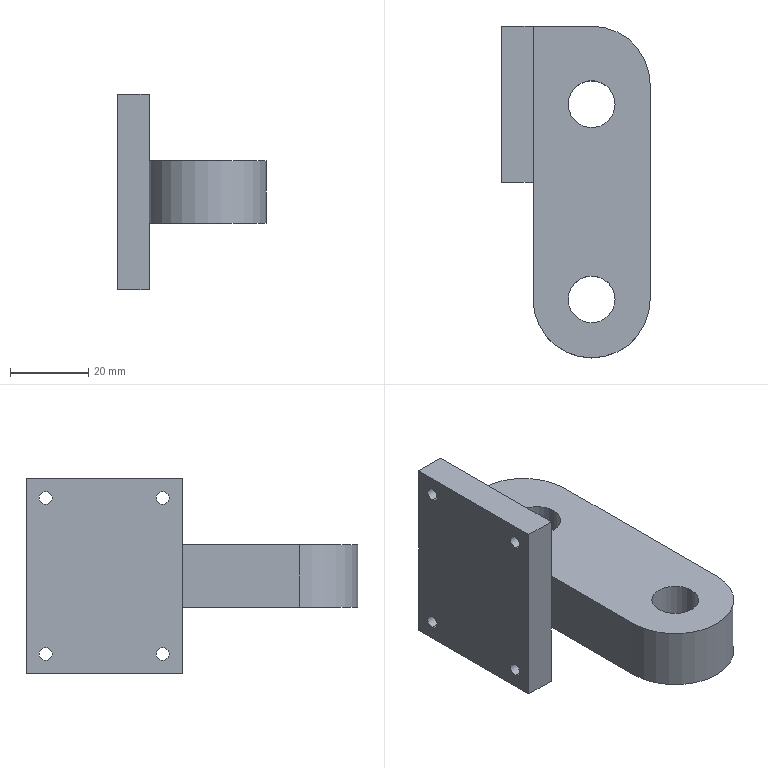Part | STEP file | X77-03303 | 1 solid | 25 faces | box 38 x 85 x 50 mm | volume 50589 mm3 | cylinder 14 | plane 11 | commonest cylinder face diameters 3.3 x8 12 x4 30 x2
STEP:
#1=CARTESIAN_POINT('',(98.602,105.281,26.35));
#2=VERTEX_POINT('',#1);
#3=CARTESIAN_POINT('',(98.602,105.281,29.65));
#4=VERTEX_POINT('',#3);
#5=CARTESIAN_POINT('',(98.602,105.281,28.));
#6=DIRECTION('',(-1.,0.,0.));
#7=DIRECTION('',(0.,0.,1.));
#8=AXIS2_PLACEMENT_3D('',#5,#6,#7);
#9=CIRCLE('',#8,1.65);
#10=EDGE_CURVE('',#2,#4,#9,.T.);
#11=ORIENTED_EDGE('',*,*,#10,.F.);
#12=CARTESIAN_POINT('',(90.602,105.281,26.35));
#13=VERTEX_POINT('',#12);
#14=CARTESIAN_POINT('',(90.602,105.281,26.35));
#15=DIRECTION('',(-1.,0.,0.));
#16=VECTOR('',#15,1000.);
#17=LINE('',#14,#16);
#18=EDGE_CURVE('',#2,#13,#17,.T.);
#19=ORIENTED_EDGE('',*,*,#18,.T.);
#20=CARTESIAN_POINT('',(90.602,105.281,29.65));
#21=VERTEX_POINT('',#20);
#22=CARTESIAN_POINT('',(90.602,105.281,28.));
#23=DIRECTION('',(-1.,0.,0.));
#24=DIRECTION('',(0.,0.,1.));
#25=AXIS2_PLACEMENT_3D('',#22,#23,#24);
#26=CIRCLE('',#25,1.65);
#27=EDGE_CURVE('',#13,#21,#26,.T.);
#28=ORIENTED_EDGE('',*,*,#27,.T.);
#29=CARTESIAN_POINT('',(90.602,105.281,29.65));
#30=DIRECTION('',(-1.,0.,0.));
#31=VECTOR('',#30,1000.);
#32=LINE('',#29,#31);
#33=EDGE_CURVE('',#4,#21,#32,.T.);
#34=ORIENTED_EDGE('',*,*,#33,.F.);
#35=EDGE_LOOP('',(#11,#19,#28,#34));
#36=FACE_OUTER_BOUND('',#35,.T.);
#37=CARTESIAN_POINT('',(90.602,105.281,28.));
#38=DIRECTION('',(-1.,0.,0.));
#39=DIRECTION('',(0.,0.,1.));
#40=AXIS2_PLACEMENT_3D('',#37,#38,#39);
#41=CYLINDRICAL_SURFACE('',#40,1.65);
#42=ADVANCED_FACE('',(#36),#41,.F.);
#43=CARTESIAN_POINT('',(98.602,105.281,-13.65));
#44=VERTEX_POINT('',#43);
#45=CARTESIAN_POINT('',(98.602,105.281,-10.35));
#46=VERTEX_POINT('',#45);
#47=CARTESIAN_POINT('',(98.602,105.281,-12.));
#48=DIRECTION('',(-1.,0.,0.));
#49=DIRECTION('',(0.,0.,1.));
#50=AXIS2_PLACEMENT_3D('',#47,#48,#49);
#51=CIRCLE('',#50,1.65);
#52=EDGE_CURVE('',#44,#46,#51,.T.);
#53=ORIENTED_EDGE('',*,*,#52,.F.);
#54=CARTESIAN_POINT('',(90.602,105.281,-13.65));
#55=VERTEX_POINT('',#54);
#56=CARTESIAN_POINT('',(90.602,105.281,-13.65));
#57=DIRECTION('',(-1.,0.,0.));
#58=VECTOR('',#57,1000.);
#59=LINE('',#56,#58);
#60=EDGE_CURVE('',#44,#55,#59,.T.);
#61=ORIENTED_EDGE('',*,*,#60,.T.);
#62=CARTESIAN_POINT('',(90.602,105.281,-10.35));
#63=VERTEX_POINT('',#62);
#64=CARTESIAN_POINT('',(90.602,105.281,-12.));
#65=DIRECTION('',(-1.,0.,0.));
#66=DIRECTION('',(0.,0.,1.));
#67=AXIS2_PLACEMENT_3D('',#64,#65,#66);
#68=CIRCLE('',#67,1.65);
#69=EDGE_CURVE('',#55,#63,#68,.T.);
#70=ORIENTED_EDGE('',*,*,#69,.T.);
#71=CARTESIAN_POINT('',(90.602,105.281,-10.35));
#72=DIRECTION('',(-1.,0.,0.));
#73=VECTOR('',#72,1000.);
#74=LINE('',#71,#73);
#75=EDGE_CURVE('',#46,#63,#74,.T.);
#76=ORIENTED_EDGE('',*,*,#75,.F.);
#77=EDGE_LOOP('',(#53,#61,#70,#76));
#78=FACE_OUTER_BOUND('',#77,.T.);
#79=CARTESIAN_POINT('',(90.602,105.281,-12.));
#80=DIRECTION('',(-1.,0.,0.));
#81=DIRECTION('',(0.,0.,1.));
#82=AXIS2_PLACEMENT_3D('',#79,#80,#81);
#83=CYLINDRICAL_SURFACE('',#82,1.65);
#84=ADVANCED_FACE('',(#78),#83,.F.);
#85=CARTESIAN_POINT('',(98.602,75.281,26.35));
#86=VERTEX_POINT('',#85);
#87=CARTESIAN_POINT('',(98.602,75.281,29.65));
#88=VERTEX_POINT('',#87);
#89=CARTESIAN_POINT('',(98.602,75.281,28.));
#90=DIRECTION('',(-1.,0.,0.));
#91=DIRECTION('',(0.,0.,1.));
#92=AXIS2_PLACEMENT_3D('',#89,#90,#91);
#93=CIRCLE('',#92,1.65);
#94=EDGE_CURVE('',#86,#88,#93,.T.);
#95=ORIENTED_EDGE('',*,*,#94,.F.);
#96=CARTESIAN_POINT('',(90.602,75.281,26.35));
#97=VERTEX_POINT('',#96);
#98=CARTESIAN_POINT('',(90.602,75.281,26.35));
#99=DIRECTION('',(-1.,0.,0.));
#100=VECTOR('',#99,1000.);
#101=LINE('',#98,#100);
#102=EDGE_CURVE('',#86,#97,#101,.T.);
#103=ORIENTED_EDGE('',*,*,#102,.T.);
#104=CARTESIAN_POINT('',(90.602,75.281,29.65));
#105=VERTEX_POINT('',#104);
#106=CARTESIAN_POINT('',(90.602,75.281,28.));
#107=DIRECTION('',(-1.,0.,0.));
#108=DIRECTION('',(0.,0.,1.));
#109=AXIS2_PLACEMENT_3D('',#106,#107,#108);
#110=CIRCLE('',#109,1.65);
#111=EDGE_CURVE('',#97,#105,#110,.T.);
#112=ORIENTED_EDGE('',*,*,#111,.T.);
#113=CARTESIAN_POINT('',(90.602,75.281,29.65));
#114=DIRECTION('',(-1.,0.,0.));
#115=VECTOR('',#114,1000.);
#116=LINE('',#113,#115);
#117=EDGE_CURVE('',#88,#105,#116,.T.);
#118=ORIENTED_EDGE('',*,*,#117,.F.);
#119=EDGE_LOOP('',(#95,#103,#112,#118));
#120=FACE_OUTER_BOUND('',#119,.T.);
#121=CARTESIAN_POINT('',(90.602,75.281,28.));
#122=DIRECTION('',(-1.,0.,0.));
#123=DIRECTION('',(0.,0.,1.));
#124=AXIS2_PLACEMENT_3D('',#121,#122,#123);
#125=CYLINDRICAL_SURFACE('',#124,1.65);
#126=ADVANCED_FACE('',(#120),#125,.F.);
#127=CARTESIAN_POINT('',(98.602,75.281,-13.65));
#128=VERTEX_POINT('',#127);
#129=CARTESIAN_POINT('',(98.602,75.281,-10.35));
#130=VERTEX_POINT('',#129);
#131=CARTESIAN_POINT('',(98.602,75.281,-12.));
#132=DIRECTION('',(-1.,0.,0.));
#133=DIRECTION('',(0.,0.,1.));
#134=AXIS2_PLACEMENT_3D('',#131,#132,#133);
#135=CIRCLE('',#134,1.65);
#136=EDGE_CURVE('',#128,#130,#135,.T.);
#137=ORIENTED_EDGE('',*,*,#136,.F.);
#138=CARTESIAN_POINT('',(90.602,75.281,-13.65));
#139=VERTEX_POINT('',#138);
#140=CARTESIAN_POINT('',(90.602,75.281,-13.65));
#141=DIRECTION('',(-1.,0.,0.));
#142=VECTOR('',#141,1000.);
#143=LINE('',#140,#142);
#144=EDGE_CURVE('',#128,#139,#143,.T.);
#145=ORIENTED_EDGE('',*,*,#144,.T.);
#146=CARTESIAN_POINT('',(90.602,75.281,-10.35));
#147=VERTEX_POINT('',#146);
#148=CARTESIAN_POINT('',(90.602,75.281,-12.));
#149=DIRECTION('',(-1.,0.,0.));
#150=DIRECTION('',(0.,0.,1.));
#151=AXIS2_PLACEMENT_3D('',#148,#149,#150);
#152=CIRCLE('',#151,1.65);
#153=EDGE_CURVE('',#139,#147,#152,.T.);
#154=ORIENTED_EDGE('',*,*,#153,.T.);
#155=CARTESIAN_POINT('',(90.602,75.281,-10.35));
#156=DIRECTION('',(-1.,0.,0.));
#157=VECTOR('',#156,1000.);
#158=LINE('',#155,#157);
#159=EDGE_CURVE('',#130,#147,#158,.T.);
#160=ORIENTED_EDGE('',*,*,#159,.F.);
#161=EDGE_LOOP('',(#137,#145,#154,#160));
#162=FACE_OUTER_BOUND('',#161,.T.);
#163=CARTESIAN_POINT('',(90.602,75.281,-12.));
#164=DIRECTION('',(-1.,0.,0.));
#165=DIRECTION('',(0.,0.,1.));
#166=AXIS2_PLACEMENT_3D('',#163,#164,#165);
#167=CYLINDRICAL_SURFACE('',#166,1.65);
#168=ADVANCED_FACE('',(#162),#167,.F.);
#169=CARTESIAN_POINT('',(107.602,90.281,16.));
#170=VERTEX_POINT('',#169);
#171=CARTESIAN_POINT('',(119.602,90.281,16.));
#172=VERTEX_POINT('',#171);
#173=CARTESIAN_POINT('',(113.602,90.281,16.));
#174=DIRECTION('',(0.,0.,1.));
#175=DIRECTION('',(1.,0.,0.));
#176=AXIS2_PLACEMENT_3D('',#173,#174,#175);
#177=CIRCLE('',#176,6.);
#178=EDGE_CURVE('',#170,#172,#177,.T.);
#179=ORIENTED_EDGE('',*,*,#178,.T.);
#180=CARTESIAN_POINT('',(119.602,90.281,0.));
#181=VERTEX_POINT('',#180);
#182=CARTESIAN_POINT('',(119.602,90.281,16.));
#183=DIRECTION('',(0.,0.,-1.));
#184=VECTOR('',#183,1000.);
#185=LINE('',#182,#184);
#186=EDGE_CURVE('',#172,#181,#185,.T.);
#187=ORIENTED_EDGE('',*,*,#186,.T.);
#188=CARTESIAN_POINT('',(107.602,90.281,0.));
#189=VERTEX_POINT('',#188);
#190=CARTESIAN_POINT('',(113.602,90.281,0.));
#191=DIRECTION('',(0.,0.,1.));
#192=DIRECTION('',(1.,0.,0.));
#193=AXIS2_PLACEMENT_3D('',#190,#191,#192);
#194=CIRCLE('',#193,6.);
#195=EDGE_CURVE('',#189,#181,#194,.T.);
#196=ORIENTED_EDGE('',*,*,#195,.F.);
#197=CARTESIAN_POINT('',(107.602,90.281,16.));
#198=DIRECTION('',(0.,0.,-1.));
#199=VECTOR('',#198,1000.);
#200=LINE('',#197,#199);
#201=EDGE_CURVE('',#170,#189,#200,.T.);
#202=ORIENTED_EDGE('',*,*,#201,.F.);
#203=EDGE_LOOP('',(#179,#187,#196,#202));
#204=FACE_OUTER_BOUND('',#203,.T.);
#205=CARTESIAN_POINT('',(113.602,90.281,16.));
#206=DIRECTION('',(0.,0.,-1.));
#207=DIRECTION('',(-1.,0.,0.));
#208=AXIS2_PLACEMENT_3D('',#205,#206,#207);
#209=CYLINDRICAL_SURFACE('',#208,6.);
#210=ADVANCED_FACE('',(#204),#209,.F.);
#211=CARTESIAN_POINT('',(107.602,40.281,16.));
#212=VERTEX_POINT('',#211);
#213=CARTESIAN_POINT('',(119.602,40.281,16.));
#214=VERTEX_POINT('',#213);
#215=CARTESIAN_POINT('',(113.602,40.281,16.));
#216=DIRECTION('',(0.,0.,1.));
#217=DIRECTION('',(1.,0.,0.));
#218=AXIS2_PLACEMENT_3D('',#215,#216,#217);
#219=CIRCLE('',#218,6.);
#220=EDGE_CURVE('',#212,#214,#219,.T.);
#221=ORIENTED_EDGE('',*,*,#220,.T.);
#222=CARTESIAN_POINT('',(119.602,40.281,0.));
#223=VERTEX_POINT('',#222);
#224=CARTESIAN_POINT('',(119.602,40.281,16.));
#225=DIRECTION('',(0.,0.,-1.));
#226=VECTOR('',#225,1000.);
#227=LINE('',#224,#226);
#228=EDGE_CURVE('',#214,#223,#227,.T.);
#229=ORIENTED_EDGE('',*,*,#228,.T.);
#230=CARTESIAN_POINT('',(107.602,40.281,0.));
#231=VERTEX_POINT('',#230);
#232=CARTESIAN_POINT('',(113.602,40.281,0.));
#233=DIRECTION('',(0.,0.,1.));
#234=DIRECTION('',(1.,0.,0.));
#235=AXIS2_PLACEMENT_3D('',#232,#233,#234);
#236=CIRCLE('',#235,6.);
#237=EDGE_CURVE('',#231,#223,#236,.T.);
#238=ORIENTED_EDGE('',*,*,#237,.F.);
#239=CARTESIAN_POINT('',(107.602,40.281,16.));
#240=DIRECTION('',(0.,0.,-1.));
#241=VECTOR('',#240,1000.);
#242=LINE('',#239,#241);
#243=EDGE_CURVE('',#212,#231,#242,.T.);
#244=ORIENTED_EDGE('',*,*,#243,.F.);
#245=EDGE_LOOP('',(#221,#229,#238,#244));
#246=FACE_OUTER_BOUND('',#245,.T.);
#247=CARTESIAN_POINT('',(113.602,40.281,16.));
#248=DIRECTION('',(0.,0.,-1.));
#249=DIRECTION('',(-1.,0.,0.));
#250=AXIS2_PLACEMENT_3D('',#247,#248,#249);
#251=CYLINDRICAL_SURFACE('',#250,6.);
#252=ADVANCED_FACE('',(#246),#251,.F.);
#253=CARTESIAN_POINT('',(98.602,70.281,0.));
#254=VERTEX_POINT('',#253);
#255=CARTESIAN_POINT('',(98.602,70.281,16.));
#256=VERTEX_POINT('',#255);
#257=CARTESIAN_POINT('',(98.602,70.281,16.));
#258=DIRECTION('',(0.,0.,1.));
#259=VECTOR('',#258,1000.);
#260=LINE('',#257,#259);
#261=EDGE_CURVE('',#254,#256,#260,.T.);
#262=ORIENTED_EDGE('',*,*,#261,.F.);
#263=CARTESIAN_POINT('',(98.602,40.281,0.));
#264=VERTEX_POINT('',#263);
#265=CARTESIAN_POINT('',(98.602,40.281,0.));
#266=DIRECTION('',(0.,-1.,0.));
#267=VECTOR('',#266,1000.);
#268=LINE('',#265,#267);
#269=EDGE_CURVE('',#254,#264,#268,.T.);
#270=ORIENTED_EDGE('',*,*,#269,.T.);
#271=CARTESIAN_POINT('',(98.602,40.281,16.));
#272=VERTEX_POINT('',#271);
#273=CARTESIAN_POINT('',(98.602,40.281,16.));
#274=DIRECTION('',(0.,0.,-1.));
#275=VECTOR('',#274,1000.);
#276=LINE('',#273,#275);
#277=EDGE_CURVE('',#272,#264,#276,.T.);
#278=ORIENTED_EDGE('',*,*,#277,.F.);
#279=CARTESIAN_POINT('',(98.602,40.281,16.));
#280=DIRECTION('',(0.,-1.,0.));
#281=VECTOR('',#280,1000.);
#282=LINE('',#279,#281);
#283=EDGE_CURVE('',#256,#272,#282,.T.);
#284=ORIENTED_EDGE('',*,*,#283,.F.);
#285=EDGE_LOOP('',(#262,#270,#278,#284));
#286=FACE_OUTER_BOUND('',#285,.T.);
#287=CARTESIAN_POINT('',(98.602,40.281,16.));
#288=DIRECTION('',(1.,0.,0.));
#289=DIRECTION('',(0.,0.,-1.));
#290=AXIS2_PLACEMENT_3D('',#287,#288,#289);
#291=PLANE('',#290);
#292=ADVANCED_FACE('',(#286),#291,.F.);
#293=ORIENTED_EDGE('',*,*,#220,.F.);
#294=CARTESIAN_POINT('',(113.602,40.281,16.));
#295=DIRECTION('',(0.,0.,1.));
#296=DIRECTION('',(1.,0.,0.));
#297=AXIS2_PLACEMENT_3D('',#294,#295,#296);
#298=CIRCLE('',#297,6.);
#299=EDGE_CURVE('',#214,#212,#298,.T.);
#300=ORIENTED_EDGE('',*,*,#299,.F.);
#301=EDGE_LOOP('',(#293,#300));
#302=FACE_BOUND('',#301,.T.);
#303=CARTESIAN_POINT('',(128.602,40.281,16.));
#304=VERTEX_POINT('',#303);
#305=CARTESIAN_POINT('',(128.602,95.281,16.));
#306=VERTEX_POINT('',#305);
#307=CARTESIAN_POINT('',(128.602,40.281,16.));
#308=DIRECTION('',(0.,1.,0.));
#309=VECTOR('',#308,1000.);
#310=LINE('',#307,#309);
#311=EDGE_CURVE('',#304,#306,#310,.T.);
#312=ORIENTED_EDGE('',*,*,#311,.T.);
#313=CARTESIAN_POINT('',(113.602,110.281,16.));
#314=VERTEX_POINT('',#313);
#315=CARTESIAN_POINT('',(113.602,95.281,16.));
#316=DIRECTION('',(0.,0.,1.));
#317=DIRECTION('',(1.,0.,0.));
#318=AXIS2_PLACEMENT_3D('',#315,#316,#317);
#319=CIRCLE('',#318,15.);
#320=EDGE_CURVE('',#306,#314,#319,.T.);
#321=ORIENTED_EDGE('',*,*,#320,.T.);
#322=CARTESIAN_POINT('',(98.602,110.281,16.));
#323=VERTEX_POINT('',#322);
#324=CARTESIAN_POINT('',(98.602,110.281,16.));
#325=DIRECTION('',(-1.,0.,0.));
#326=VECTOR('',#325,1000.);
#327=LINE('',#324,#326);
#328=EDGE_CURVE('',#314,#323,#327,.T.);
#329=ORIENTED_EDGE('',*,*,#328,.T.);
#330=CARTESIAN_POINT('',(98.602,40.281,16.));
#331=DIRECTION('',(0.,-1.,0.));
#332=VECTOR('',#331,1000.);
#333=LINE('',#330,#332);
#334=EDGE_CURVE('',#323,#256,#333,.T.);
#335=ORIENTED_EDGE('',*,*,#334,.T.);
#336=ORIENTED_EDGE('',*,*,#283,.T.);
#337=CARTESIAN_POINT('',(113.602,40.281,16.));
#338=DIRECTION('',(0.,0.,1.));
#339=DIRECTION('',(1.,0.,0.));
#340=AXIS2_PLACEMENT_3D('',#337,#338,#339);
#341=CIRCLE('',#340,15.);
#342=EDGE_CURVE('',#272,#304,#341,.T.);
#343=ORIENTED_EDGE('',*,*,#342,.T.);
#344=EDGE_LOOP('',(#312,#321,#329,#335,#336,#343));
#345=FACE_OUTER_BOUND('',#344,.T.);
#346=ORIENTED_EDGE('',*,*,#178,.F.);
#347=CARTESIAN_POINT('',(113.602,90.281,16.));
#348=DIRECTION('',(0.,0.,1.));
#349=DIRECTION('',(1.,0.,0.));
#350=AXIS2_PLACEMENT_3D('',#347,#348,#349);
#351=CIRCLE('',#350,6.);
#352=EDGE_CURVE('',#172,#170,#351,.T.);
#353=ORIENTED_EDGE('',*,*,#352,.F.);
#354=EDGE_LOOP('',(#346,#353));
#355=FACE_BOUND('',#354,.T.);
#356=CARTESIAN_POINT('',(113.602,40.281,16.));
#357=DIRECTION('',(0.,0.,1.));
#358=DIRECTION('',(1.,0.,0.));
#359=AXIS2_PLACEMENT_3D('',#356,#357,#358);
#360=PLANE('',#359);
#361=ADVANCED_FACE('',(#302,#345,#355),#360,.T.);
#362=ORIENTED_EDGE('',*,*,#237,.T.);
#363=CARTESIAN_POINT('',(113.602,40.281,0.));
#364=DIRECTION('',(0.,0.,1.));
#365=DIRECTION('',(1.,0.,0.));
#366=AXIS2_PLACEMENT_3D('',#363,#364,#365);
#367=CIRCLE('',#366,6.);
#368=EDGE_CURVE('',#223,#231,#367,.T.);
#369=ORIENTED_EDGE('',*,*,#368,.T.);
#370=EDGE_LOOP('',(#362,#369));
#371=FACE_BOUND('',#370,.T.);
#372=CARTESIAN_POINT('',(113.602,110.281,0.));
#373=VERTEX_POINT('',#372);
#374=CARTESIAN_POINT('',(98.602,110.281,0.));
#375=VERTEX_POINT('',#374);
#376=CARTESIAN_POINT('',(98.602,110.281,0.));
#377=DIRECTION('',(-1.,0.,0.));
#378=VECTOR('',#377,1000.);
#379=LINE('',#376,#378);
#380=EDGE_CURVE('',#373,#375,#379,.T.);
#381=ORIENTED_EDGE('',*,*,#380,.F.);
#382=CARTESIAN_POINT('',(128.602,95.281,0.));
#383=VERTEX_POINT('',#382);
#384=CARTESIAN_POINT('',(113.602,95.281,0.));
#385=DIRECTION('',(0.,0.,-1.));
#386=DIRECTION('',(1.,0.,0.));
#387=AXIS2_PLACEMENT_3D('',#384,#385,#386);
#388=CIRCLE('',#387,15.);
#389=EDGE_CURVE('',#373,#383,#388,.T.);
#390=ORIENTED_EDGE('',*,*,#389,.T.);
#391=CARTESIAN_POINT('',(128.602,40.281,0.));
#392=VERTEX_POINT('',#391);
#393=CARTESIAN_POINT('',(128.602,40.281,0.));
#394=DIRECTION('',(0.,1.,0.));
#395=VECTOR('',#394,1000.);
#396=LINE('',#393,#395);
#397=EDGE_CURVE('',#392,#383,#396,.T.);
#398=ORIENTED_EDGE('',*,*,#397,.F.);
#399=CARTESIAN_POINT('',(113.602,40.281,0.));
#400=DIRECTION('',(0.,0.,1.));
#401=DIRECTION('',(1.,0.,0.));
#402=AXIS2_PLACEMENT_3D('',#399,#400,#401);
#403=CIRCLE('',#402,15.);
#404=EDGE_CURVE('',#264,#392,#403,.T.);
#405=ORIENTED_EDGE('',*,*,#404,.F.);
#406=ORIENTED_EDGE('',*,*,#269,.F.);
#407=CARTESIAN_POINT('',(98.602,40.281,0.));
#408=DIRECTION('',(0.,-1.,0.));
#409=VECTOR('',#408,1000.);
#410=LINE('',#407,#409);
#411=EDGE_CURVE('',#375,#254,#410,.T.);
#412=ORIENTED_EDGE('',*,*,#411,.F.);
#413=EDGE_LOOP('',(#381,#390,#398,#405,#406,#412));
#414=FACE_OUTER_BOUND('',#413,.T.);
#415=ORIENTED_EDGE('',*,*,#195,.T.);
#416=CARTESIAN_POINT('',(113.602,90.281,0.));
#417=DIRECTION('',(0.,0.,1.));
#418=DIRECTION('',(1.,0.,0.));
#419=AXIS2_PLACEMENT_3D('',#416,#417,#418);
#420=CIRCLE('',#419,6.);
#421=EDGE_CURVE('',#181,#189,#420,.T.);
#422=ORIENTED_EDGE('',*,*,#421,.T.);
#423=EDGE_LOOP('',(#415,#422));
#424=FACE_BOUND('',#423,.T.);
#425=CARTESIAN_POINT('',(113.602,40.281,0.));
#426=DIRECTION('',(0.,0.,1.));
#427=DIRECTION('',(1.,0.,0.));
#428=AXIS2_PLACEMENT_3D('',#425,#426,#427);
#429=PLANE('',#428);
#430=ADVANCED_FACE('',(#371,#414,#424),#429,.F.);
#431=ORIENTED_EDGE('',*,*,#404,.T.);
#432=CARTESIAN_POINT('',(128.602,40.281,16.));
#433=DIRECTION('',(0.,0.,-1.));
#434=VECTOR('',#433,1000.);
#435=LINE('',#432,#434);
#436=EDGE_CURVE('',#304,#392,#435,.T.);
#437=ORIENTED_EDGE('',*,*,#436,.F.);
#438=ORIENTED_EDGE('',*,*,#342,.F.);
#439=ORIENTED_EDGE('',*,*,#277,.T.);
#440=EDGE_LOOP('',(#431,#437,#438,#439));
#441=FACE_OUTER_BOUND('',#440,.T.);
#442=CARTESIAN_POINT('',(113.602,40.281,16.));
#443=DIRECTION('',(0.,0.,-1.));
#444=DIRECTION('',(-1.,0.,0.));
#445=AXIS2_PLACEMENT_3D('',#442,#443,#444);
#446=CYLINDRICAL_SURFACE('',#445,15.);
#447=ADVANCED_FACE('',(#441),#446,.T.);
#448=ORIENTED_EDGE('',*,*,#397,.T.);
#449=CARTESIAN_POINT('',(128.602,95.281,16.));
#450=DIRECTION('',(0.,0.,1.));
#451=VECTOR('',#450,1000.);
#452=LINE('',#449,#451);
#453=EDGE_CURVE('',#383,#306,#452,.T.);
#454=ORIENTED_EDGE('',*,*,#453,.T.);
#455=ORIENTED_EDGE('',*,*,#311,.F.);
#456=ORIENTED_EDGE('',*,*,#436,.T.);
#457=EDGE_LOOP('',(#448,#454,#455,#456));
#458=FACE_OUTER_BOUND('',#457,.T.);
#459=CARTESIAN_POINT('',(128.602,40.281,16.));
#460=DIRECTION('',(-1.,0.,0.));
#461=DIRECTION('',(0.,-1.,0.));
#462=AXIS2_PLACEMENT_3D('',#459,#460,#461);
#463=PLANE('',#462);
#464=ADVANCED_FACE('',(#458),#463,.F.);
#465=ORIENTED_EDGE('',*,*,#328,.F.);
#466=CARTESIAN_POINT('',(113.602,110.281,16.));
#467=DIRECTION('',(0.,0.,-1.));
#468=VECTOR('',#467,1000.);
#469=LINE('',#466,#468);
#470=EDGE_CURVE('',#314,#373,#469,.T.);
#471=ORIENTED_EDGE('',*,*,#470,.T.);
#472=ORIENTED_EDGE('',*,*,#380,.T.);
#473=CARTESIAN_POINT('',(98.602,110.281,-17.));
#474=VERTEX_POINT('',#473);
#475=CARTESIAN_POINT('',(98.602,110.281,-17.));
#476=DIRECTION('',(0.,0.,-1.));
#477=VECTOR('',#476,1000.);
#478=LINE('',#475,#477);
#479=EDGE_CURVE('',#375,#474,#478,.T.);
#480=ORIENTED_EDGE('',*,*,#479,.T.);
#481=CARTESIAN_POINT('',(90.602,110.281,-17.));
#482=VERTEX_POINT('',#481);
#483=CARTESIAN_POINT('',(90.602,110.281,-17.));
#484=DIRECTION('',(1.,0.,0.));
#485=VECTOR('',#484,1000.);
#486=LINE('',#483,#485);
#487=EDGE_CURVE('',#482,#474,#486,.T.);
#488=ORIENTED_EDGE('',*,*,#487,.F.);
#489=CARTESIAN_POINT('',(90.602,110.281,33.));
#490=VERTEX_POINT('',#489);
#491=CARTESIAN_POINT('',(90.602,110.281,-17.));
#492=DIRECTION('',(0.,0.,-1.));
#493=VECTOR('',#492,1000.);
#494=LINE('',#491,#493);
#495=EDGE_CURVE('',#490,#482,#494,.T.);
#496=ORIENTED_EDGE('',*,*,#495,.F.);
#497=CARTESIAN_POINT('',(98.602,110.281,33.));
#498=VERTEX_POINT('',#497);
#499=CARTESIAN_POINT('',(90.602,110.281,33.));
#500=DIRECTION('',(1.,0.,0.));
#501=VECTOR('',#500,1000.);
#502=LINE('',#499,#501);
#503=EDGE_CURVE('',#490,#498,#502,.T.);
#504=ORIENTED_EDGE('',*,*,#503,.T.);
#505=CARTESIAN_POINT('',(98.602,110.281,-17.));
#506=DIRECTION('',(0.,0.,-1.));
#507=VECTOR('',#506,1000.);
#508=LINE('',#505,#507);
#509=EDGE_CURVE('',#498,#323,#508,.T.);
#510=ORIENTED_EDGE('',*,*,#509,.T.);
#511=EDGE_LOOP('',(#465,#471,#472,#480,#488,#496,#504,#510));
#512=FACE_OUTER_BOUND('',#511,.T.);
#513=CARTESIAN_POINT('',(98.602,110.281,16.));
#514=DIRECTION('',(0.,-1.,0.));
#515=DIRECTION('',(0.,0.,-1.));
#516=AXIS2_PLACEMENT_3D('',#513,#514,#515);
#517=PLANE('',#516);
#518=ADVANCED_FACE('',(#512),#517,.F.);
#519=ORIENTED_EDGE('',*,*,#228,.F.);
#520=ORIENTED_EDGE('',*,*,#299,.T.);
#521=ORIENTED_EDGE('',*,*,#243,.T.);
#522=ORIENTED_EDGE('',*,*,#368,.F.);
#523=EDGE_LOOP('',(#519,#520,#521,#522));
#524=FACE_OUTER_BOUND('',#523,.T.);
#525=CARTESIAN_POINT('',(113.602,40.281,16.));
#526=DIRECTION('',(0.,0.,-1.));
#527=DIRECTION('',(-1.,0.,0.));
#528=AXIS2_PLACEMENT_3D('',#525,#526,#527);
#529=CYLINDRICAL_SURFACE('',#528,6.);
#530=ADVANCED_FACE('',(#524),#529,.F.);
#531=ORIENTED_EDGE('',*,*,#186,.F.);
#532=ORIENTED_EDGE('',*,*,#352,.T.);
#533=ORIENTED_EDGE('',*,*,#201,.T.);
#534=ORIENTED_EDGE('',*,*,#421,.F.);
#535=EDGE_LOOP('',(#531,#532,#533,#534));
#536=FACE_OUTER_BOUND('',#535,.T.);
#537=CARTESIAN_POINT('',(113.602,90.281,16.));
#538=DIRECTION('',(0.,0.,-1.));
#539=DIRECTION('',(-1.,0.,0.));
#540=AXIS2_PLACEMENT_3D('',#537,#538,#539);
#541=CYLINDRICAL_SURFACE('',#540,6.);
#542=ADVANCED_FACE('',(#536),#541,.F.);
#543=CARTESIAN_POINT('',(98.602,105.281,-12.));
#544=DIRECTION('',(-1.,0.,0.));
#545=DIRECTION('',(0.,0.,1.));
#546=AXIS2_PLACEMENT_3D('',#543,#544,#545);
#547=CIRCLE('',#546,1.65);
#548=EDGE_CURVE('',#46,#44,#547,.T.);
#549=ORIENTED_EDGE('',*,*,#548,.T.);
#550=ORIENTED_EDGE('',*,*,#52,.T.);
#551=EDGE_LOOP('',(#549,#550));
#552=FACE_BOUND('',#551,.T.);
#553=CARTESIAN_POINT('',(98.602,75.281,-12.));
#554=DIRECTION('',(-1.,0.,0.));
#555=DIRECTION('',(0.,0.,1.));
#556=AXIS2_PLACEMENT_3D('',#553,#554,#555);
#557=CIRCLE('',#556,1.65);
#558=EDGE_CURVE('',#130,#128,#557,.T.);
#559=ORIENTED_EDGE('',*,*,#558,.T.);
#560=ORIENTED_EDGE('',*,*,#136,.T.);
#561=EDGE_LOOP('',(#559,#560));
#562=FACE_BOUND('',#561,.T.);
#563=ORIENTED_EDGE('',*,*,#479,.F.);
#564=ORIENTED_EDGE('',*,*,#411,.T.);
#565=CARTESIAN_POINT('',(98.602,70.281,-17.));
#566=VERTEX_POINT('',#565);
#567=CARTESIAN_POINT('',(98.602,70.281,-17.));
#568=DIRECTION('',(0.,0.,1.));
#569=VECTOR('',#568,1000.);
#570=LINE('',#567,#569);
#571=EDGE_CURVE('',#566,#254,#570,.T.);
#572=ORIENTED_EDGE('',*,*,#571,.F.);
#573=CARTESIAN_POINT('',(98.602,110.281,-17.));
#574=DIRECTION('',(0.,-1.,0.));
#575=VECTOR('',#574,1000.);
#576=LINE('',#573,#575);
#577=EDGE_CURVE('',#474,#566,#576,.T.);
#578=ORIENTED_EDGE('',*,*,#577,.F.);
#579=EDGE_LOOP('',(#563,#564,#572,#578));
#580=FACE_OUTER_BOUND('',#579,.T.);
#581=CARTESIAN_POINT('',(98.602,70.281,-17.));
#582=DIRECTION('',(-1.,0.,0.));
#583=DIRECTION('',(0.,0.,1.));
#584=AXIS2_PLACEMENT_3D('',#581,#582,#583);
#585=PLANE('',#584);
#586=ADVANCED_FACE('',(#552,#562,#580),#585,.F.);
#587=ORIENTED_EDGE('',*,*,#577,.T.);
#588=CARTESIAN_POINT('',(90.602,70.281,-17.));
#589=VERTEX_POINT('',#588);
#590=CARTESIAN_POINT('',(90.602,70.281,-17.));
#591=DIRECTION('',(1.,0.,0.));
#592=VECTOR('',#591,1000.);
#593=LINE('',#590,#592);
#594=EDGE_CURVE('',#589,#566,#593,.T.);
#595=ORIENTED_EDGE('',*,*,#594,.F.);
#596=CARTESIAN_POINT('',(90.602,110.281,-17.));
#597=DIRECTION('',(0.,-1.,0.));
#598=VECTOR('',#597,1000.);
#599=LINE('',#596,#598);
#600=EDGE_CURVE('',#482,#589,#599,.T.);
#601=ORIENTED_EDGE('',*,*,#600,.F.);
#602=ORIENTED_EDGE('',*,*,#487,.T.);
#603=EDGE_LOOP('',(#587,#595,#601,#602));
#604=FACE_OUTER_BOUND('',#603,.T.);
#605=CARTESIAN_POINT('',(90.602,110.281,-17.));
#606=DIRECTION('',(0.,0.,1.));
#607=DIRECTION('',(0.,-1.,0.));
#608=AXIS2_PLACEMENT_3D('',#605,#606,#607);
#609=PLANE('',#608);
#610=ADVANCED_FACE('',(#604),#609,.F.);
#611=ORIENTED_EDGE('',*,*,#571,.T.);
#612=ORIENTED_EDGE('',*,*,#261,.T.);
#613=CARTESIAN_POINT('',(98.602,70.281,33.));
#614=VERTEX_POINT('',#613);
#615=CARTESIAN_POINT('',(98.602,70.281,-17.));
#616=DIRECTION('',(0.,0.,1.));
#617=VECTOR('',#616,1000.);
#618=LINE('',#615,#617);
#619=EDGE_CURVE('',#256,#614,#618,.T.);
#620=ORIENTED_EDGE('',*,*,#619,.T.);
#621=CARTESIAN_POINT('',(90.602,70.281,33.));
#622=VERTEX_POINT('',#621);
#623=CARTESIAN_POINT('',(90.602,70.281,33.));
#624=DIRECTION('',(1.,0.,0.));
#625=VECTOR('',#624,1000.);
#626=LINE('',#623,#625);
#627=EDGE_CURVE('',#622,#614,#626,.T.);
#628=ORIENTED_EDGE('',*,*,#627,.F.);
#629=CARTESIAN_POINT('',(90.602,70.281,-17.));
#630=DIRECTION('',(0.,0.,1.));
#631=VECTOR('',#630,1000.);
#632=LINE('',#629,#631);
#633=EDGE_CURVE('',#589,#622,#632,.T.);
#634=ORIENTED_EDGE('',*,*,#633,.F.);
#635=ORIENTED_EDGE('',*,*,#594,.T.);
#636=EDGE_LOOP('',(#611,#612,#620,#628,#634,#635));
#637=FACE_OUTER_BOUND('',#636,.T.);
#638=CARTESIAN_POINT('',(90.602,70.281,-17.));
#639=DIRECTION('',(0.,1.,0.));
#640=DIRECTION('',(0.,0.,1.));
#641=AXIS2_PLACEMENT_3D('',#638,#639,#640);
#642=PLANE('',#641);
#643=ADVANCED_FACE('',(#637),#642,.F.);
#644=CARTESIAN_POINT('',(98.602,110.281,33.));
#645=DIRECTION('',(0.,1.,0.));
#646=VECTOR('',#645,1000.);
#647=LINE('',#644,#646);
#648=EDGE_CURVE('',#614,#498,#647,.T.);
#649=ORIENTED_EDGE('',*,*,#648,.T.);
#650=ORIENTED_EDGE('',*,*,#503,.F.);
#651=CARTESIAN_POINT('',(90.602,110.281,33.));
#652=DIRECTION('',(0.,1.,0.));
#653=VECTOR('',#652,1000.);
#654=LINE('',#651,#653);
#655=EDGE_CURVE('',#622,#490,#654,.T.);
#656=ORIENTED_EDGE('',*,*,#655,.F.);
#657=ORIENTED_EDGE('',*,*,#627,.T.);
#658=EDGE_LOOP('',(#649,#650,#656,#657));
#659=FACE_OUTER_BOUND('',#658,.T.);
#660=CARTESIAN_POINT('',(90.602,110.281,33.));
#661=DIRECTION('',(0.,0.,-1.));
#662=DIRECTION('',(0.,1.,0.));
#663=AXIS2_PLACEMENT_3D('',#660,#661,#662);
#664=PLANE('',#663);
#665=ADVANCED_FACE('',(#659),#664,.F.);
#666=CARTESIAN_POINT('',(90.602,105.281,28.));
#667=DIRECTION('',(-1.,0.,0.));
#668=DIRECTION('',(0.,0.,1.));
#669=AXIS2_PLACEMENT_3D('',#666,#667,#668);
#670=CIRCLE('',#669,1.65);
#671=EDGE_CURVE('',#21,#13,#670,.T.);
#672=ORIENTED_EDGE('',*,*,#671,.F.);
#673=ORIENTED_EDGE('',*,*,#27,.F.);
#674=EDGE_LOOP('',(#672,#673));
#675=FACE_BOUND('',#674,.T.);
#676=CARTESIAN_POINT('',(90.602,105.281,-12.));
#677=DIRECTION('',(-1.,0.,0.));
#678=DIRECTION('',(0.,0.,1.));
#679=AXIS2_PLACEMENT_3D('',#676,#677,#678);
#680=CIRCLE('',#679,1.65);
#681=EDGE_CURVE('',#63,#55,#680,.T.);
#682=ORIENTED_EDGE('',*,*,#681,.F.);
#683=ORIENTED_EDGE('',*,*,#69,.F.);
#684=EDGE_LOOP('',(#682,#683));
#685=FACE_BOUND('',#684,.T.);
#686=CARTESIAN_POINT('',(90.602,75.281,28.));
#687=DIRECTION('',(-1.,0.,0.));
#688=DIRECTION('',(0.,0.,1.));
#689=AXIS2_PLACEMENT_3D('',#686,#687,#688);
#690=CIRCLE('',#689,1.65);
#691=EDGE_CURVE('',#105,#97,#690,.T.);
#692=ORIENTED_EDGE('',*,*,#691,.F.);
#693=ORIENTED_EDGE('',*,*,#111,.F.);
#694=EDGE_LOOP('',(#692,#693));
#695=FACE_BOUND('',#694,.T.);
#696=CARTESIAN_POINT('',(90.602,75.281,-12.));
#697=DIRECTION('',(-1.,0.,0.));
#698=DIRECTION('',(0.,0.,1.));
#699=AXIS2_PLACEMENT_3D('',#696,#697,#698);
#700=CIRCLE('',#699,1.65);
#701=EDGE_CURVE('',#147,#139,#700,.T.);
#702=ORIENTED_EDGE('',*,*,#701,.F.);
#703=ORIENTED_EDGE('',*,*,#153,.F.);
#704=EDGE_LOOP('',(#702,#703));
#705=FACE_BOUND('',#704,.T.);
#706=ORIENTED_EDGE('',*,*,#600,.T.);
#707=ORIENTED_EDGE('',*,*,#633,.T.);
#708=ORIENTED_EDGE('',*,*,#655,.T.);
#709=ORIENTED_EDGE('',*,*,#495,.T.);
#710=EDGE_LOOP('',(#706,#707,#708,#709));
#711=FACE_OUTER_BOUND('',#710,.T.);
#712=CARTESIAN_POINT('',(90.602,70.281,-17.));
#713=DIRECTION('',(-1.,0.,0.));
#714=DIRECTION('',(0.,0.,1.));
#715=AXIS2_PLACEMENT_3D('',#712,#713,#714);
#716=PLANE('',#715);
#717=ADVANCED_FACE('',(#675,#685,#695,#705,#711),#716,.T.);
#718=CARTESIAN_POINT('',(98.602,105.281,28.));
#719=DIRECTION('',(-1.,0.,0.));
#720=DIRECTION('',(0.,0.,1.));
#721=AXIS2_PLACEMENT_3D('',#718,#719,#720);
#722=CIRCLE('',#721,1.65);
#723=EDGE_CURVE('',#4,#2,#722,.T.);
#724=ORIENTED_EDGE('',*,*,#723,.T.);
#725=ORIENTED_EDGE('',*,*,#10,.T.);
#726=EDGE_LOOP('',(#724,#725));
#727=FACE_BOUND('',#726,.T.);
#728=CARTESIAN_POINT('',(98.602,75.281,28.));
#729=DIRECTION('',(-1.,0.,0.));
#730=DIRECTION('',(0.,0.,1.));
#731=AXIS2_PLACEMENT_3D('',#728,#729,#730);
#732=CIRCLE('',#731,1.65);
#733=EDGE_CURVE('',#88,#86,#732,.T.);
#734=ORIENTED_EDGE('',*,*,#733,.T.);
#735=ORIENTED_EDGE('',*,*,#94,.T.);
#736=EDGE_LOOP('',(#734,#735));
#737=FACE_BOUND('',#736,.T.);
#738=ORIENTED_EDGE('',*,*,#334,.F.);
#739=ORIENTED_EDGE('',*,*,#509,.F.);
#740=ORIENTED_EDGE('',*,*,#648,.F.);
#741=ORIENTED_EDGE('',*,*,#619,.F.);
#742=EDGE_LOOP('',(#738,#739,#740,#741));
#743=FACE_OUTER_BOUND('',#742,.T.);
#744=CARTESIAN_POINT('',(98.602,70.281,-17.));
#745=DIRECTION('',(-1.,0.,0.));
#746=DIRECTION('',(0.,0.,1.));
#747=AXIS2_PLACEMENT_3D('',#744,#745,#746);
#748=PLANE('',#747);
#749=ADVANCED_FACE('',(#727,#737,#743),#748,.F.);
#750=ORIENTED_EDGE('',*,*,#320,.F.);
#751=ORIENTED_EDGE('',*,*,#453,.F.);
#752=ORIENTED_EDGE('',*,*,#389,.F.);
#753=ORIENTED_EDGE('',*,*,#470,.F.);
#754=EDGE_LOOP('',(#750,#751,#752,#753));
#755=FACE_OUTER_BOUND('',#754,.T.);
#756=CARTESIAN_POINT('',(113.602,95.281,16.));
#757=DIRECTION('',(0.,0.,-1.));
#758=DIRECTION('',(-1.,0.,0.));
#759=AXIS2_PLACEMENT_3D('',#756,#757,#758);
#760=CYLINDRICAL_SURFACE('',#759,15.);
#761=ADVANCED_FACE('',(#755),#760,.T.);
#762=ORIENTED_EDGE('',*,*,#144,.F.);
#763=ORIENTED_EDGE('',*,*,#558,.F.);
#764=ORIENTED_EDGE('',*,*,#159,.T.);
#765=ORIENTED_EDGE('',*,*,#701,.T.);
#766=EDGE_LOOP('',(#762,#763,#764,#765));
#767=FACE_OUTER_BOUND('',#766,.T.);
#768=CARTESIAN_POINT('',(90.602,75.281,-12.));
#769=DIRECTION('',(-1.,0.,0.));
#770=DIRECTION('',(0.,0.,1.));
#771=AXIS2_PLACEMENT_3D('',#768,#769,#770);
#772=CYLINDRICAL_SURFACE('',#771,1.65);
#773=ADVANCED_FACE('',(#767),#772,.F.);
#774=ORIENTED_EDGE('',*,*,#102,.F.);
#775=ORIENTED_EDGE('',*,*,#733,.F.);
#776=ORIENTED_EDGE('',*,*,#117,.T.);
#777=ORIENTED_EDGE('',*,*,#691,.T.);
#778=EDGE_LOOP('',(#774,#775,#776,#777));
#779=FACE_OUTER_BOUND('',#778,.T.);
#780=CARTESIAN_POINT('',(90.602,75.281,28.));
#781=DIRECTION('',(-1.,0.,0.));
#782=DIRECTION('',(0.,0.,1.));
#783=AXIS2_PLACEMENT_3D('',#780,#781,#782);
#784=CYLINDRICAL_SURFACE('',#783,1.65);
#785=ADVANCED_FACE('',(#779),#784,.F.);
#786=ORIENTED_EDGE('',*,*,#60,.F.);
#787=ORIENTED_EDGE('',*,*,#548,.F.);
#788=ORIENTED_EDGE('',*,*,#75,.T.);
#789=ORIENTED_EDGE('',*,*,#681,.T.);
#790=EDGE_LOOP('',(#786,#787,#788,#789));
#791=FACE_OUTER_BOUND('',#790,.T.);
#792=CARTESIAN_POINT('',(90.602,105.281,-12.));
#793=DIRECTION('',(-1.,0.,0.));
#794=DIRECTION('',(0.,0.,1.));
#795=AXIS2_PLACEMENT_3D('',#792,#793,#794);
#796=CYLINDRICAL_SURFACE('',#795,1.65);
#797=ADVANCED_FACE('',(#791),#796,.F.);
#798=ORIENTED_EDGE('',*,*,#18,.F.);
#799=ORIENTED_EDGE('',*,*,#723,.F.);
#800=ORIENTED_EDGE('',*,*,#33,.T.);
#801=ORIENTED_EDGE('',*,*,#671,.T.);
#802=EDGE_LOOP('',(#798,#799,#800,#801));
#803=FACE_OUTER_BOUND('',#802,.T.);
#804=CARTESIAN_POINT('',(90.602,105.281,28.));
#805=DIRECTION('',(-1.,0.,0.));
#806=DIRECTION('',(0.,0.,1.));
#807=AXIS2_PLACEMENT_3D('',#804,#805,#806);
#808=CYLINDRICAL_SURFACE('',#807,1.65);
#809=ADVANCED_FACE('',(#803),#808,.F.);
#810=CLOSED_SHELL('',(#42,#84,#126,#168,#210,#252,#292,#361,#430,#447,#464,#518,#530,#542,#586,#610,#643,#665,#717,#749,#761,#773,#785,#797,#809));
#811=MANIFOLD_SOLID_BREP('',#810);
#812=CARTESIAN_POINT('',(0.,0.,0.));
#813=DIRECTION('',(0.,0.,1.));
#814=DIRECTION('',(1.,0.,0.));
#815=AXIS2_PLACEMENT_3D('',#812,#813,#814);
#816=(LENGTH_UNIT()NAMED_UNIT(*)SI_UNIT(.MILLI.,.METRE.));
#817=UNCERTAINTY_MEASURE_WITH_UNIT(LENGTH_MEASURE(0.00001),#816,'','');
#818=(NAMED_UNIT(*)PLANE_ANGLE_UNIT()SI_UNIT($,.RADIAN.));
#819=(NAMED_UNIT(*)SI_UNIT($,.STERADIAN.)SOLID_ANGLE_UNIT());
#820=(GEOMETRIC_REPRESENTATION_CONTEXT(3)GLOBAL_UNCERTAINTY_ASSIGNED_CONTEXT((#817))GLOBAL_UNIT_ASSIGNED_CONTEXT((#816,#818,#819))REPRESENTATION_CONTEXT('',''));
#821=ADVANCED_BREP_SHAPE_REPRESENTATION('',(#811,#815),#820);